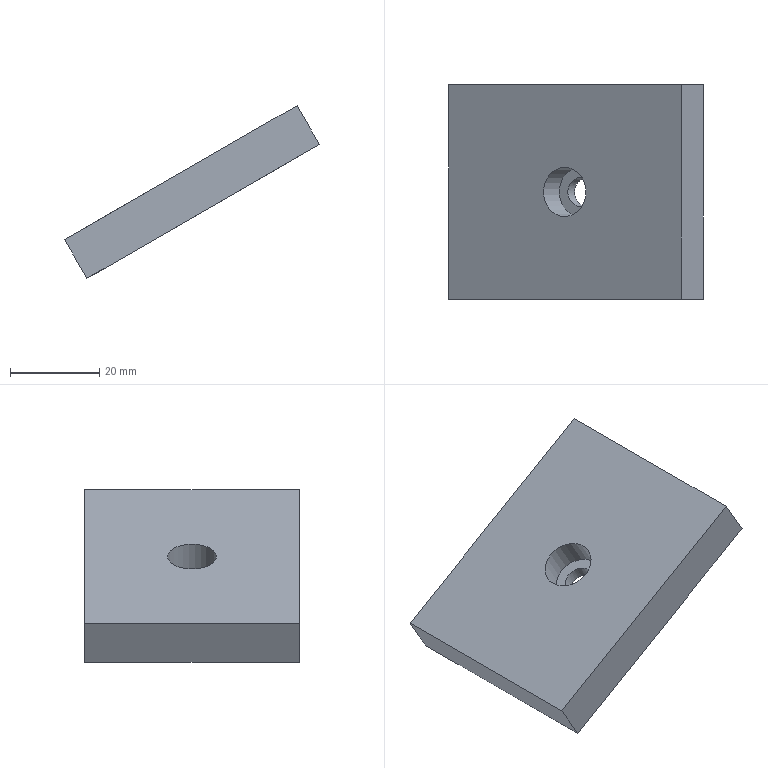Part | STEP file | solid 2 | 1 solid | 9 faces | box 56.962 x 48 x 38.66 mm | volume 28035 mm3 | plane 7 | cylinder 2 | commonest cylinder face diameters 6.5 x1 11 x1